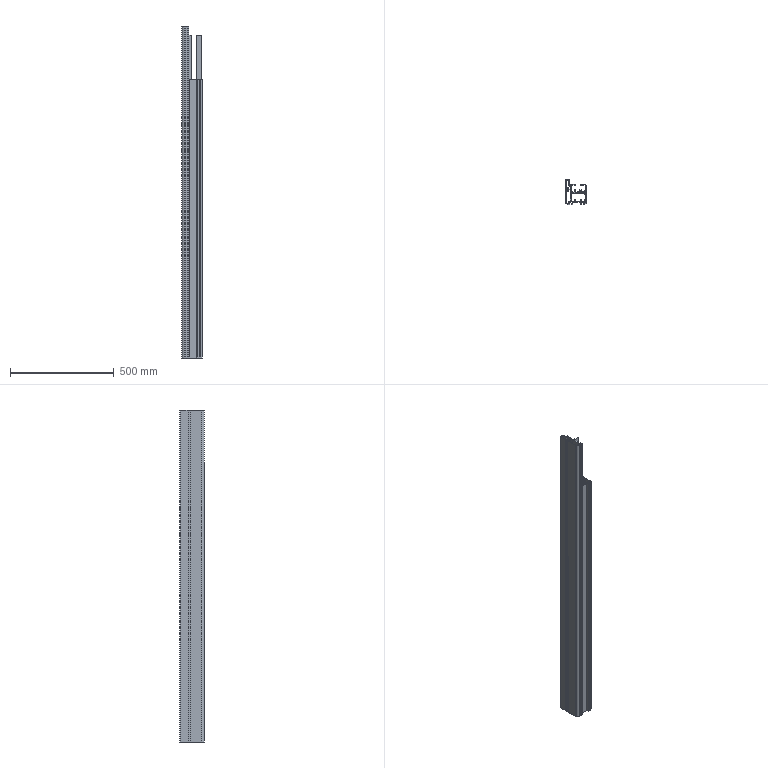Part | STEP file | PN_0007_default | 1 solid | 212 faces | box 100 x 118 x 1600 mm | volume 2634824 mm3 | plane 128 | cylinder 84 | commonest cylinder face diameters 1 x56 4 x22 2 x2 10 x1 16 x1 20 x1